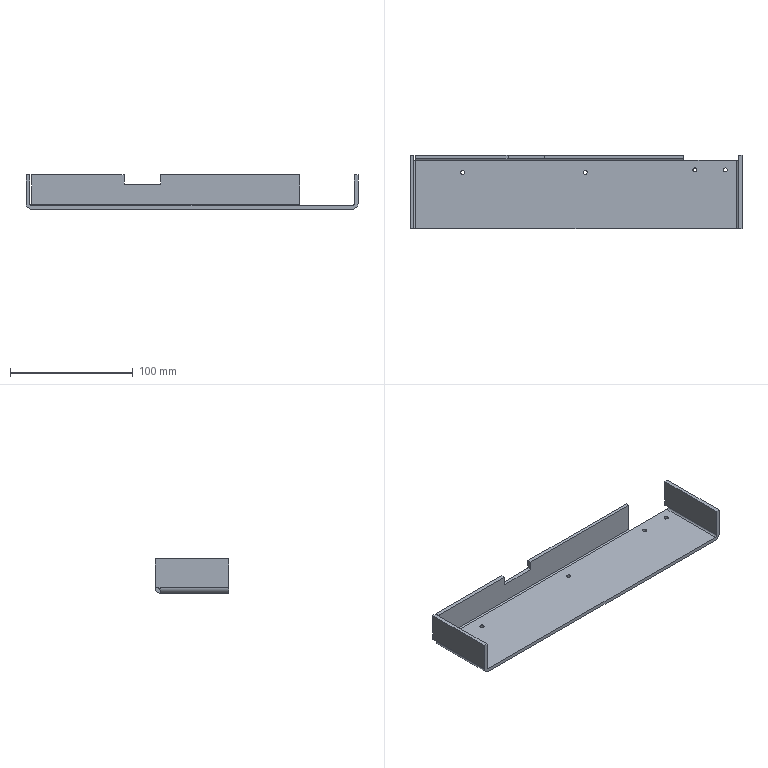Part | NX | features BREP 1 | 1 solid | 34 faces | box 271 x 60 x 28 mm | volume 71630 mm3 | plane 24 | cylinder 10 | commonest cylinder face diameters 3.3 x4 3 x2 9 x2 2 x1 8 x1
STEP:
#1=CARTESIAN_POINT('',(139.15,18.,0.));
#2=VERTEX_POINT('',#1);
#3=CARTESIAN_POINT('',(137.5,18.,0.));
#4=DIRECTION('',(0.,0.,1.));
#5=DIRECTION('',(1.,0.,0.));
#6=AXIS2_PLACEMENT_3D('',#3,#4,#5);
#7=CIRCLE('',#6,1.65);
#8=EDGE_CURVE('',#2,#2,#7,.T.);
#9=ORIENTED_EDGE('',*,*,#8,.T.);
#10=EDGE_LOOP('',(#9));
#11=FACE_BOUND('',#10,.T.);
#12=CARTESIAN_POINT('',(139.15,18.,-3.));
#13=VERTEX_POINT('',#12);
#14=CARTESIAN_POINT('',(137.5,18.,-3.));
#15=DIRECTION('',(0.,0.,1.));
#16=DIRECTION('',(1.,0.,0.));
#17=AXIS2_PLACEMENT_3D('',#14,#15,#16);
#18=CIRCLE('',#17,1.65);
#19=EDGE_CURVE('',#13,#13,#18,.T.);
#20=ORIENTED_EDGE('',*,*,#19,.F.);
#21=EDGE_LOOP('',(#20));
#22=FACE_BOUND('',#21,.T.);
#23=CARTESIAN_POINT('',(137.5,18.,0.));
#24=DIRECTION('',(0.,0.,1.));
#25=DIRECTION('',(1.,0.,0.));
#26=AXIS2_PLACEMENT_3D('',#23,#24,#25);
#27=CYLINDRICAL_SURFACE('',#26,1.65);
#28=ADVANCED_FACE('',(#11,#22),#27,.F.);
#29=CARTESIAN_POINT('',(164.15,18.,0.));
#30=VERTEX_POINT('',#29);
#31=CARTESIAN_POINT('',(162.5,18.,0.));
#32=DIRECTION('',(0.,0.,1.));
#33=DIRECTION('',(1.,0.,0.));
#34=AXIS2_PLACEMENT_3D('',#31,#32,#33);
#35=CIRCLE('',#34,1.65);
#36=EDGE_CURVE('',#30,#30,#35,.T.);
#37=ORIENTED_EDGE('',*,*,#36,.T.);
#38=EDGE_LOOP('',(#37));
#39=FACE_BOUND('',#38,.T.);
#40=CARTESIAN_POINT('',(164.15,18.,-3.));
#41=VERTEX_POINT('',#40);
#42=CARTESIAN_POINT('',(162.5,18.,-3.));
#43=DIRECTION('',(0.,0.,1.));
#44=DIRECTION('',(1.,0.,0.));
#45=AXIS2_PLACEMENT_3D('',#42,#43,#44);
#46=CIRCLE('',#45,1.65);
#47=EDGE_CURVE('',#41,#41,#46,.T.);
#48=ORIENTED_EDGE('',*,*,#47,.F.);
#49=EDGE_LOOP('',(#48));
#50=FACE_BOUND('',#49,.T.);
#51=CARTESIAN_POINT('',(162.5,18.,0.));
#52=DIRECTION('',(0.,0.,1.));
#53=DIRECTION('',(1.,0.,0.));
#54=AXIS2_PLACEMENT_3D('',#51,#52,#53);
#55=CYLINDRICAL_SURFACE('',#54,1.65);
#56=ADVANCED_FACE('',(#39,#50),#55,.F.);
#57=CARTESIAN_POINT('',(49.65,16.,0.));
#58=VERTEX_POINT('',#57);
#59=CARTESIAN_POINT('',(48.,16.,0.));
#60=DIRECTION('',(0.,0.,1.));
#61=DIRECTION('',(1.,0.,0.));
#62=AXIS2_PLACEMENT_3D('',#59,#60,#61);
#63=CIRCLE('',#62,1.65);
#64=EDGE_CURVE('',#58,#58,#63,.T.);
#65=ORIENTED_EDGE('',*,*,#64,.T.);
#66=EDGE_LOOP('',(#65));
#67=FACE_BOUND('',#66,.T.);
#68=CARTESIAN_POINT('',(49.65,16.,-3.));
#69=VERTEX_POINT('',#68);
#70=CARTESIAN_POINT('',(48.,16.,-3.));
#71=DIRECTION('',(0.,0.,1.));
#72=DIRECTION('',(1.,0.,0.));
#73=AXIS2_PLACEMENT_3D('',#70,#71,#72);
#74=CIRCLE('',#73,1.65);
#75=EDGE_CURVE('',#69,#69,#74,.T.);
#76=ORIENTED_EDGE('',*,*,#75,.F.);
#77=EDGE_LOOP('',(#76));
#78=FACE_BOUND('',#77,.T.);
#79=CARTESIAN_POINT('',(48.,16.,0.));
#80=DIRECTION('',(0.,0.,1.));
#81=DIRECTION('',(1.,0.,0.));
#82=AXIS2_PLACEMENT_3D('',#79,#80,#81);
#83=CYLINDRICAL_SURFACE('',#82,1.65);
#84=ADVANCED_FACE('',(#67,#78),#83,.F.);
#85=CARTESIAN_POINT('',(-50.35,16.,0.));
#86=VERTEX_POINT('',#85);
#87=CARTESIAN_POINT('',(-52.,16.,0.));
#88=DIRECTION('',(0.,0.,1.));
#89=DIRECTION('',(1.,0.,0.));
#90=AXIS2_PLACEMENT_3D('',#87,#88,#89);
#91=CIRCLE('',#90,1.65);
#92=EDGE_CURVE('',#86,#86,#91,.T.);
#93=ORIENTED_EDGE('',*,*,#92,.T.);
#94=EDGE_LOOP('',(#93));
#95=FACE_BOUND('',#94,.T.);
#96=CARTESIAN_POINT('',(-50.35,16.,-3.));
#97=VERTEX_POINT('',#96);
#98=CARTESIAN_POINT('',(-52.,16.,-3.));
#99=DIRECTION('',(0.,0.,1.));
#100=DIRECTION('',(1.,0.,0.));
#101=AXIS2_PLACEMENT_3D('',#98,#99,#100);
#102=CIRCLE('',#101,1.65);
#103=EDGE_CURVE('',#97,#97,#102,.T.);
#104=ORIENTED_EDGE('',*,*,#103,.F.);
#105=EDGE_LOOP('',(#104));
#106=FACE_BOUND('',#105,.T.);
#107=CARTESIAN_POINT('',(-52.,16.,0.));
#108=DIRECTION('',(0.,0.,1.));
#109=DIRECTION('',(1.,0.,0.));
#110=AXIS2_PLACEMENT_3D('',#107,#108,#109);
#111=CYLINDRICAL_SURFACE('',#110,1.65);
#112=ADVANCED_FACE('',(#95,#106),#111,.F.);
#113=CARTESIAN_POINT('',(128.5,30.,1.));
#114=VERTEX_POINT('',#113);
#115=CARTESIAN_POINT('',(-90.5,30.,1.));
#116=VERTEX_POINT('',#115);
#117=CARTESIAN_POINT('',(0.,30.,1.));
#118=DIRECTION('',(-1.,0.,0.));
#119=VECTOR('',#118,1000.);
#120=LINE('',#117,#119);
#121=EDGE_CURVE('',#114,#116,#120,.T.);
#122=ORIENTED_EDGE('',*,*,#121,.F.);
#123=CARTESIAN_POINT('',(128.5,26.,-3.));
#124=VERTEX_POINT('',#123);
#125=CARTESIAN_POINT('',(128.5,26.,1.));
#126=DIRECTION('',(1.,0.,0.));
#127=DIRECTION('',(0.,-1.,0.));
#128=AXIS2_PLACEMENT_3D('',#125,#126,#127);
#129=CIRCLE('',#128,4.);
#130=EDGE_CURVE('',#124,#114,#129,.T.);
#131=ORIENTED_EDGE('',*,*,#130,.F.);
#132=CARTESIAN_POINT('',(-90.5,26.,-3.));
#133=VERTEX_POINT('',#132);
#134=CARTESIAN_POINT('',(-90.5,26.,-3.));
#135=DIRECTION('',(1.,0.,0.));
#136=VECTOR('',#135,1000.);
#137=LINE('',#134,#136);
#138=EDGE_CURVE('',#133,#124,#137,.T.);
#139=ORIENTED_EDGE('',*,*,#138,.F.);
#140=CARTESIAN_POINT('',(-90.5,26.,1.));
#141=DIRECTION('',(-1.,0.,0.));
#142=DIRECTION('',(0.,-1.,0.));
#143=AXIS2_PLACEMENT_3D('',#140,#141,#142);
#144=CIRCLE('',#143,4.);
#145=EDGE_CURVE('',#116,#133,#144,.T.);
#146=ORIENTED_EDGE('',*,*,#145,.F.);
#147=EDGE_LOOP('',(#122,#131,#139,#146));
#148=FACE_BOUND('',#147,.T.);
#149=CARTESIAN_POINT('',(-90.5,26.,1.));
#150=DIRECTION('',(-1.,0.,0.));
#151=DIRECTION('',(0.,1.,0.));
#152=AXIS2_PLACEMENT_3D('',#149,#150,#151);
#153=CYLINDRICAL_SURFACE('',#152,4.);
#154=ADVANCED_FACE('',(#148),#153,.T.);
#155=CARTESIAN_POINT('',(128.5,26.,0.));
#156=VERTEX_POINT('',#155);
#157=CARTESIAN_POINT('',(128.5,27.,1.));
#158=VERTEX_POINT('',#157);
#159=CARTESIAN_POINT('',(128.5,26.,1.));
#160=DIRECTION('',(1.,0.,0.));
#161=DIRECTION('',(0.,0.,1.));
#162=AXIS2_PLACEMENT_3D('',#159,#160,#161);
#163=CIRCLE('',#162,1.);
#164=EDGE_CURVE('',#156,#158,#163,.T.);
#165=ORIENTED_EDGE('',*,*,#164,.T.);
#166=CARTESIAN_POINT('',(-90.5,27.,1.));
#167=VERTEX_POINT('',#166);
#168=CARTESIAN_POINT('',(171.5,27.,1.));
#169=DIRECTION('',(-1.,0.,0.));
#170=VECTOR('',#169,1000.);
#171=LINE('',#168,#170);
#172=EDGE_CURVE('',#158,#167,#171,.T.);
#173=ORIENTED_EDGE('',*,*,#172,.T.);
#174=CARTESIAN_POINT('',(-90.5,26.,0.));
#175=VERTEX_POINT('',#174);
#176=CARTESIAN_POINT('',(-90.5,26.,1.));
#177=DIRECTION('',(-1.,0.,0.));
#178=DIRECTION('',(0.,-1.,0.));
#179=AXIS2_PLACEMENT_3D('',#176,#177,#178);
#180=CIRCLE('',#179,1.);
#181=EDGE_CURVE('',#167,#175,#180,.T.);
#182=ORIENTED_EDGE('',*,*,#181,.T.);
#183=CARTESIAN_POINT('',(-90.5,26.,0.));
#184=DIRECTION('',(1.,0.,0.));
#185=VECTOR('',#184,1000.);
#186=LINE('',#183,#185);
#187=EDGE_CURVE('',#175,#156,#186,.T.);
#188=ORIENTED_EDGE('',*,*,#187,.T.);
#189=EDGE_LOOP('',(#165,#173,#182,#188));
#190=FACE_BOUND('',#189,.T.);
#191=CARTESIAN_POINT('',(-90.5,26.,1.));
#192=DIRECTION('',(-1.,0.,0.));
#193=DIRECTION('',(0.,1.,0.));
#194=AXIS2_PLACEMENT_3D('',#191,#192,#193);
#195=CYLINDRICAL_SURFACE('',#194,1.);
#196=ADVANCED_FACE('',(#190),#195,.F.);
#197=CARTESIAN_POINT('',(128.5,30.,25.));
#198=VERTEX_POINT('',#197);
#199=CARTESIAN_POINT('',(15.,30.,25.));
#200=VERTEX_POINT('',#199);
#201=CARTESIAN_POINT('',(-90.5,30.,25.));
#202=DIRECTION('',(-1.,0.,0.));
#203=VECTOR('',#202,1000.);
#204=LINE('',#201,#203);
#205=EDGE_CURVE('',#198,#200,#204,.T.);
#206=ORIENTED_EDGE('',*,*,#205,.F.);
#207=CARTESIAN_POINT('',(128.5,30.,0.));
#208=DIRECTION('',(0.,0.,1.));
#209=VECTOR('',#208,1000.);
#210=LINE('',#207,#209);
#211=EDGE_CURVE('',#114,#198,#210,.T.);
#212=ORIENTED_EDGE('',*,*,#211,.F.);
#213=ORIENTED_EDGE('',*,*,#121,.T.);
#214=CARTESIAN_POINT('',(-90.5,30.,25.));
#215=VERTEX_POINT('',#214);
#216=CARTESIAN_POINT('',(-90.5,30.,0.));
#217=DIRECTION('',(0.,0.,-1.));
#218=VECTOR('',#217,1000.);
#219=LINE('',#216,#218);
#220=EDGE_CURVE('',#215,#116,#219,.T.);
#221=ORIENTED_EDGE('',*,*,#220,.F.);
#222=CARTESIAN_POINT('',(-15.,30.,25.));
#223=VERTEX_POINT('',#222);
#224=CARTESIAN_POINT('',(-90.5,30.,25.));
#225=DIRECTION('',(-1.,0.,0.));
#226=VECTOR('',#225,1000.);
#227=LINE('',#224,#226);
#228=EDGE_CURVE('',#223,#215,#227,.T.);
#229=ORIENTED_EDGE('',*,*,#228,.F.);
#230=CARTESIAN_POINT('',(-15.,30.,17.5));
#231=VERTEX_POINT('',#230);
#232=CARTESIAN_POINT('',(-15.,30.,17.5));
#233=DIRECTION('',(0.,0.,1.));
#234=VECTOR('',#233,1000.);
#235=LINE('',#232,#234);
#236=EDGE_CURVE('',#231,#223,#235,.T.);
#237=ORIENTED_EDGE('',*,*,#236,.F.);
#238=CARTESIAN_POINT('',(15.,30.,17.5));
#239=VERTEX_POINT('',#238);
#240=CARTESIAN_POINT('',(15.,30.,17.5));
#241=DIRECTION('',(-1.,0.,0.));
#242=VECTOR('',#241,1000.);
#243=LINE('',#240,#242);
#244=EDGE_CURVE('',#239,#231,#243,.T.);
#245=ORIENTED_EDGE('',*,*,#244,.F.);
#246=CARTESIAN_POINT('',(15.,30.,17.5));
#247=DIRECTION('',(0.,0.,-1.));
#248=VECTOR('',#247,1000.);
#249=LINE('',#246,#248);
#250=EDGE_CURVE('',#200,#239,#249,.T.);
#251=ORIENTED_EDGE('',*,*,#250,.F.);
#252=EDGE_LOOP('',(#206,#212,#213,#221,#229,#237,#245,#251));
#253=FACE_BOUND('',#252,.T.);
#254=CARTESIAN_POINT('',(0.,30.,0.));
#255=DIRECTION('',(0.,1.,0.));
#256=DIRECTION('',(-1.,0.,0.));
#257=AXIS2_PLACEMENT_3D('',#254,#255,#256);
#258=PLANE('',#257);
#259=ADVANCED_FACE('',(#253),#258,.T.);
#260=CARTESIAN_POINT('',(128.5,27.,25.));
#261=VERTEX_POINT('',#260);
#262=CARTESIAN_POINT('',(128.5,27.,0.));
#263=DIRECTION('',(0.,0.,1.));
#264=VECTOR('',#263,1000.);
#265=LINE('',#262,#264);
#266=EDGE_CURVE('',#158,#261,#265,.T.);
#267=ORIENTED_EDGE('',*,*,#266,.T.);
#268=CARTESIAN_POINT('',(15.,27.,25.));
#269=VERTEX_POINT('',#268);
#270=CARTESIAN_POINT('',(0.,27.,25.));
#271=DIRECTION('',(-1.,0.,0.));
#272=VECTOR('',#271,1000.);
#273=LINE('',#270,#272);
#274=EDGE_CURVE('',#261,#269,#273,.T.);
#275=ORIENTED_EDGE('',*,*,#274,.T.);
#276=CARTESIAN_POINT('',(15.,27.,17.5));
#277=VERTEX_POINT('',#276);
#278=CARTESIAN_POINT('',(15.,27.,0.));
#279=DIRECTION('',(0.,0.,-1.));
#280=VECTOR('',#279,1000.);
#281=LINE('',#278,#280);
#282=EDGE_CURVE('',#269,#277,#281,.T.);
#283=ORIENTED_EDGE('',*,*,#282,.T.);
#284=CARTESIAN_POINT('',(-15.,27.,17.5));
#285=VERTEX_POINT('',#284);
#286=CARTESIAN_POINT('',(0.,27.,17.5));
#287=DIRECTION('',(-1.,0.,0.));
#288=VECTOR('',#287,1000.);
#289=LINE('',#286,#288);
#290=EDGE_CURVE('',#277,#285,#289,.T.);
#291=ORIENTED_EDGE('',*,*,#290,.T.);
#292=CARTESIAN_POINT('',(-15.,27.,25.));
#293=VERTEX_POINT('',#292);
#294=CARTESIAN_POINT('',(-15.,27.,0.));
#295=DIRECTION('',(0.,0.,1.));
#296=VECTOR('',#295,1000.);
#297=LINE('',#294,#296);
#298=EDGE_CURVE('',#285,#293,#297,.T.);
#299=ORIENTED_EDGE('',*,*,#298,.T.);
#300=CARTESIAN_POINT('',(-90.5,27.,25.));
#301=VERTEX_POINT('',#300);
#302=CARTESIAN_POINT('',(0.,27.,25.));
#303=DIRECTION('',(-1.,0.,0.));
#304=VECTOR('',#303,1000.);
#305=LINE('',#302,#304);
#306=EDGE_CURVE('',#293,#301,#305,.T.);
#307=ORIENTED_EDGE('',*,*,#306,.T.);
#308=CARTESIAN_POINT('',(-90.5,27.,0.));
#309=DIRECTION('',(0.,0.,-1.));
#310=VECTOR('',#309,1000.);
#311=LINE('',#308,#310);
#312=EDGE_CURVE('',#301,#167,#311,.T.);
#313=ORIENTED_EDGE('',*,*,#312,.T.);
#314=ORIENTED_EDGE('',*,*,#172,.F.);
#315=EDGE_LOOP('',(#267,#275,#283,#291,#299,#307,#313,#314));
#316=FACE_BOUND('',#315,.T.);
#317=CARTESIAN_POINT('',(0.,27.,0.));
#318=DIRECTION('',(0.,1.,0.));
#319=DIRECTION('',(-1.,0.,0.));
#320=AXIS2_PLACEMENT_3D('',#317,#318,#319);
#321=PLANE('',#320);
#322=ADVANCED_FACE('',(#316),#321,.F.);
#323=ORIENTED_EDGE('',*,*,#274,.F.);
#324=CARTESIAN_POINT('',(128.5,27.,25.));
#325=DIRECTION('',(0.,1.,0.));
#326=VECTOR('',#325,1000.);
#327=LINE('',#324,#326);
#328=EDGE_CURVE('',#261,#198,#327,.T.);
#329=ORIENTED_EDGE('',*,*,#328,.T.);
#330=ORIENTED_EDGE('',*,*,#205,.T.);
#331=CARTESIAN_POINT('',(15.,30.,25.));
#332=DIRECTION('',(0.,1.,0.));
#333=VECTOR('',#332,1000.);
#334=LINE('',#331,#333);
#335=EDGE_CURVE('',#269,#200,#334,.T.);
#336=ORIENTED_EDGE('',*,*,#335,.F.);
#337=EDGE_LOOP('',(#323,#329,#330,#336));
#338=FACE_BOUND('',#337,.T.);
#339=CARTESIAN_POINT('',(-90.5,30.,25.));
#340=DIRECTION('',(0.,0.,1.));
#341=DIRECTION('',(0.,-1.,0.));
#342=AXIS2_PLACEMENT_3D('',#339,#340,#341);
#343=PLANE('',#342);
#344=ADVANCED_FACE('',(#338),#343,.T.);
#345=CARTESIAN_POINT('',(-15.,30.,25.));
#346=DIRECTION('',(0.,-1.,0.));
#347=VECTOR('',#346,1000.);
#348=LINE('',#345,#347);
#349=EDGE_CURVE('',#223,#293,#348,.T.);
#350=ORIENTED_EDGE('',*,*,#349,.F.);
#351=ORIENTED_EDGE('',*,*,#228,.T.);
#352=CARTESIAN_POINT('',(-90.5,30.,25.));
#353=DIRECTION('',(0.,-1.,0.));
#354=VECTOR('',#353,1000.);
#355=LINE('',#352,#354);
#356=EDGE_CURVE('',#215,#301,#355,.T.);
#357=ORIENTED_EDGE('',*,*,#356,.T.);
#358=ORIENTED_EDGE('',*,*,#306,.F.);
#359=EDGE_LOOP('',(#350,#351,#357,#358));
#360=FACE_BOUND('',#359,.T.);
#361=CARTESIAN_POINT('',(-90.5,30.,25.));
#362=DIRECTION('',(0.,0.,1.));
#363=DIRECTION('',(0.,-1.,0.));
#364=AXIS2_PLACEMENT_3D('',#361,#362,#363);
#365=PLANE('',#364);
#366=ADVANCED_FACE('',(#360),#365,.T.);
#367=CARTESIAN_POINT('',(-95.,26.,1.5));
#368=VERTEX_POINT('',#367);
#369=CARTESIAN_POINT('',(-92.,26.,1.5));
#370=VERTEX_POINT('',#369);
#371=CARTESIAN_POINT('',(-95.,26.,1.5));
#372=DIRECTION('',(1.,0.,0.));
#373=VECTOR('',#372,1000.);
#374=LINE('',#371,#373);
#375=EDGE_CURVE('',#368,#370,#374,.T.);
#376=ORIENTED_EDGE('',*,*,#375,.F.);
#377=CARTESIAN_POINT('',(-95.,30.,1.5));
#378=VERTEX_POINT('',#377);
#379=CARTESIAN_POINT('',(-95.,30.,1.5));
#380=DIRECTION('',(0.,1.,0.));
#381=VECTOR('',#380,1000.);
#382=LINE('',#379,#381);
#383=EDGE_CURVE('',#368,#378,#382,.T.);
#384=ORIENTED_EDGE('',*,*,#383,.T.);
#385=CARTESIAN_POINT('',(-92.,30.,1.5));
#386=VERTEX_POINT('',#385);
#387=CARTESIAN_POINT('',(-95.,30.,1.5));
#388=DIRECTION('',(-1.,0.,0.));
#389=VECTOR('',#388,1000.);
#390=LINE('',#387,#389);
#391=EDGE_CURVE('',#386,#378,#390,.T.);
#392=ORIENTED_EDGE('',*,*,#391,.F.);
#393=CARTESIAN_POINT('',(-92.,30.,1.5));
#394=DIRECTION('',(0.,-1.,0.));
#395=VECTOR('',#394,1000.);
#396=LINE('',#393,#395);
#397=EDGE_CURVE('',#386,#370,#396,.T.);
#398=ORIENTED_EDGE('',*,*,#397,.T.);
#399=EDGE_LOOP('',(#376,#384,#392,#398));
#400=FACE_BOUND('',#399,.T.);
#401=CARTESIAN_POINT('',(0.,0.,1.5));
#402=DIRECTION('',(0.,0.,-1.));
#403=DIRECTION('',(-1.,0.,0.));
#404=AXIS2_PLACEMENT_3D('',#401,#402,#403);
#405=PLANE('',#404);
#406=ADVANCED_FACE('',(#400),#405,.T.);
#407=CARTESIAN_POINT('',(-95.,-30.,1.5));
#408=VERTEX_POINT('',#407);
#409=CARTESIAN_POINT('',(-95.,30.,1.5));
#410=DIRECTION('',(0.,1.,0.));
#411=VECTOR('',#410,1000.);
#412=LINE('',#409,#411);
#413=EDGE_CURVE('',#408,#368,#412,.T.);
#414=ORIENTED_EDGE('',*,*,#413,.T.);
#415=CARTESIAN_POINT('',(-90.5,26.,1.5));
#416=DIRECTION('',(0.,-1.,0.));
#417=DIRECTION('',(0.,0.,1.));
#418=AXIS2_PLACEMENT_3D('',#415,#416,#417);
#419=CIRCLE('',#418,4.5);
#420=EDGE_CURVE('',#368,#133,#419,.T.);
#421=ORIENTED_EDGE('',*,*,#420,.T.);
#422=CARTESIAN_POINT('',(-90.5,-30.,-3.));
#423=VERTEX_POINT('',#422);
#424=CARTESIAN_POINT('',(-90.5,-30.,-3.));
#425=DIRECTION('',(0.,1.,0.));
#426=VECTOR('',#425,1000.);
#427=LINE('',#424,#426);
#428=EDGE_CURVE('',#423,#133,#427,.T.);
#429=ORIENTED_EDGE('',*,*,#428,.F.);
#430=CARTESIAN_POINT('',(-90.5,-30.,1.5));
#431=DIRECTION('',(0.,-1.,0.));
#432=DIRECTION('',(0.,0.,-1.));
#433=AXIS2_PLACEMENT_3D('',#430,#431,#432);
#434=CIRCLE('',#433,4.5);
#435=EDGE_CURVE('',#408,#423,#434,.T.);
#436=ORIENTED_EDGE('',*,*,#435,.F.);
#437=EDGE_LOOP('',(#414,#421,#429,#436));
#438=FACE_BOUND('',#437,.T.);
#439=CARTESIAN_POINT('',(-90.5,-30.,1.5));
#440=DIRECTION('',(0.,-1.,0.));
#441=DIRECTION('',(-1.,0.,0.));
#442=AXIS2_PLACEMENT_3D('',#439,#440,#441);
#443=CYLINDRICAL_SURFACE('',#442,4.5);
#444=ADVANCED_FACE('',(#438),#443,.T.);
#445=CARTESIAN_POINT('',(173.,26.,1.5));
#446=VERTEX_POINT('',#445);
#447=CARTESIAN_POINT('',(176.,26.,1.5));
#448=VERTEX_POINT('',#447);
#449=CARTESIAN_POINT('',(173.,26.,1.5));
#450=DIRECTION('',(1.,0.,0.));
#451=VECTOR('',#450,1000.);
#452=LINE('',#449,#451);
#453=EDGE_CURVE('',#446,#448,#452,.T.);
#454=ORIENTED_EDGE('',*,*,#453,.F.);
#455=CARTESIAN_POINT('',(173.,30.,1.5));
#456=VERTEX_POINT('',#455);
#457=CARTESIAN_POINT('',(173.,-30.,1.5));
#458=DIRECTION('',(0.,1.,0.));
#459=VECTOR('',#458,1000.);
#460=LINE('',#457,#459);
#461=EDGE_CURVE('',#446,#456,#460,.T.);
#462=ORIENTED_EDGE('',*,*,#461,.T.);
#463=CARTESIAN_POINT('',(176.,30.,1.5));
#464=VERTEX_POINT('',#463);
#465=CARTESIAN_POINT('',(173.,30.,1.5));
#466=DIRECTION('',(1.,0.,0.));
#467=VECTOR('',#466,1000.);
#468=LINE('',#465,#467);
#469=EDGE_CURVE('',#456,#464,#468,.T.);
#470=ORIENTED_EDGE('',*,*,#469,.T.);
#471=CARTESIAN_POINT('',(176.,-30.,1.5));
#472=DIRECTION('',(0.,-1.,0.));
#473=VECTOR('',#472,1000.);
#474=LINE('',#471,#473);
#475=EDGE_CURVE('',#464,#448,#474,.T.);
#476=ORIENTED_EDGE('',*,*,#475,.T.);
#477=EDGE_LOOP('',(#454,#462,#470,#476));
#478=FACE_BOUND('',#477,.T.);
#479=CARTESIAN_POINT('',(0.,0.,1.5));
#480=DIRECTION('',(0.,0.,1.));
#481=DIRECTION('',(1.,0.,0.));
#482=AXIS2_PLACEMENT_3D('',#479,#480,#481);
#483=PLANE('',#482);
#484=ADVANCED_FACE('',(#478),#483,.F.);
#485=CARTESIAN_POINT('',(171.5,26.,-3.));
#486=VERTEX_POINT('',#485);
#487=CARTESIAN_POINT('',(171.5,-30.,-3.));
#488=VERTEX_POINT('',#487);
#489=CARTESIAN_POINT('',(171.5,30.,-3.));
#490=DIRECTION('',(0.,-1.,0.));
#491=VECTOR('',#490,1000.);
#492=LINE('',#489,#491);
#493=EDGE_CURVE('',#486,#488,#492,.T.);
#494=ORIENTED_EDGE('',*,*,#493,.F.);
#495=CARTESIAN_POINT('',(171.5,26.,1.5));
#496=DIRECTION('',(0.,-1.,0.));
#497=DIRECTION('',(0.,0.,1.));
#498=AXIS2_PLACEMENT_3D('',#495,#496,#497);
#499=CIRCLE('',#498,4.5);
#500=EDGE_CURVE('',#486,#448,#499,.T.);
#501=ORIENTED_EDGE('',*,*,#500,.T.);
#502=CARTESIAN_POINT('',(176.,-30.,1.5));
#503=VERTEX_POINT('',#502);
#504=CARTESIAN_POINT('',(176.,-30.,1.5));
#505=DIRECTION('',(0.,-1.,0.));
#506=VECTOR('',#505,1000.);
#507=LINE('',#504,#506);
#508=EDGE_CURVE('',#448,#503,#507,.T.);
#509=ORIENTED_EDGE('',*,*,#508,.T.);
#510=CARTESIAN_POINT('',(171.5,-30.,1.5));
#511=DIRECTION('',(0.,-1.,0.));
#512=DIRECTION('',(0.,0.,1.));
#513=AXIS2_PLACEMENT_3D('',#510,#511,#512);
#514=CIRCLE('',#513,4.5);
#515=EDGE_CURVE('',#488,#503,#514,.T.);
#516=ORIENTED_EDGE('',*,*,#515,.F.);
#517=EDGE_LOOP('',(#494,#501,#509,#516));
#518=FACE_BOUND('',#517,.T.);
#519=CARTESIAN_POINT('',(171.5,30.,1.5));
#520=DIRECTION('',(0.,1.,0.));
#521=DIRECTION('',(1.,0.,0.));
#522=AXIS2_PLACEMENT_3D('',#519,#520,#521);
#523=CYLINDRICAL_SURFACE('',#522,4.5);
#524=ADVANCED_FACE('',(#518),#523,.T.);
#525=CARTESIAN_POINT('',(171.5,26.,0.));
#526=VERTEX_POINT('',#525);
#527=CARTESIAN_POINT('',(171.5,26.,1.5));
#528=DIRECTION('',(0.,-1.,0.));
#529=DIRECTION('',(0.,0.,1.));
#530=AXIS2_PLACEMENT_3D('',#527,#528,#529);
#531=CIRCLE('',#530,1.5);
#532=EDGE_CURVE('',#526,#446,#531,.T.);
#533=ORIENTED_EDGE('',*,*,#532,.T.);
#534=ORIENTED_EDGE('',*,*,#453,.T.);
#535=ORIENTED_EDGE('',*,*,#500,.F.);
#536=CARTESIAN_POINT('',(-90.5,26.,-3.));
#537=DIRECTION('',(1.,0.,0.));
#538=VECTOR('',#537,1000.);
#539=LINE('',#536,#538);
#540=EDGE_CURVE('',#124,#486,#539,.T.);
#541=ORIENTED_EDGE('',*,*,#540,.F.);
#542=CARTESIAN_POINT('',(128.5,26.,0.));
#543=DIRECTION('',(0.,0.,-1.));
#544=VECTOR('',#543,1000.);
#545=LINE('',#542,#544);
#546=EDGE_CURVE('',#156,#124,#545,.T.);
#547=ORIENTED_EDGE('',*,*,#546,.F.);
#548=CARTESIAN_POINT('',(-90.5,26.,0.));
#549=DIRECTION('',(1.,0.,0.));
#550=VECTOR('',#549,1000.);
#551=LINE('',#548,#550);
#552=EDGE_CURVE('',#156,#526,#551,.T.);
#553=ORIENTED_EDGE('',*,*,#552,.T.);
#554=EDGE_LOOP('',(#533,#534,#535,#541,#547,#553));
#555=FACE_BOUND('',#554,.T.);
#556=CARTESIAN_POINT('',(171.5,26.,1.5));
#557=DIRECTION('',(0.,1.,0.));
#558=DIRECTION('',(0.,0.,1.));
#559=AXIS2_PLACEMENT_3D('',#556,#557,#558);
#560=PLANE('',#559);
#561=ADVANCED_FACE('',(#555),#560,.T.);
#562=ORIENTED_EDGE('',*,*,#19,.T.);
#563=EDGE_LOOP('',(#562));
#564=FACE_BOUND('',#563,.T.);
#565=ORIENTED_EDGE('',*,*,#47,.T.);
#566=EDGE_LOOP('',(#565));
#567=FACE_BOUND('',#566,.T.);
#568=ORIENTED_EDGE('',*,*,#75,.T.);
#569=EDGE_LOOP('',(#568));
#570=FACE_BOUND('',#569,.T.);
#571=ORIENTED_EDGE('',*,*,#103,.T.);
#572=EDGE_LOOP('',(#571));
#573=FACE_BOUND('',#572,.T.);
#574=ORIENTED_EDGE('',*,*,#428,.T.);
#575=ORIENTED_EDGE('',*,*,#138,.T.);
#576=ORIENTED_EDGE('',*,*,#540,.T.);
#577=ORIENTED_EDGE('',*,*,#493,.T.);
#578=CARTESIAN_POINT('',(-95.,-30.,-3.));
#579=DIRECTION('',(1.,0.,0.));
#580=VECTOR('',#579,1000.);
#581=LINE('',#578,#580);
#582=EDGE_CURVE('',#423,#488,#581,.T.);
#583=ORIENTED_EDGE('',*,*,#582,.F.);
#584=EDGE_LOOP('',(#574,#575,#576,#577,#583));
#585=FACE_BOUND('',#584,.T.);
#586=CARTESIAN_POINT('',(0.,0.,-3.));
#587=DIRECTION('',(0.,0.,-1.));
#588=DIRECTION('',(-1.,0.,0.));
#589=AXIS2_PLACEMENT_3D('',#586,#587,#588);
#590=PLANE('',#589);
#591=ADVANCED_FACE('',(#564,#567,#570,#573,#585),#590,.T.);
#592=ORIENTED_EDGE('',*,*,#8,.F.);
#593=EDGE_LOOP('',(#592));
#594=FACE_BOUND('',#593,.T.);
#595=ORIENTED_EDGE('',*,*,#36,.F.);
#596=EDGE_LOOP('',(#595));
#597=FACE_BOUND('',#596,.T.);
#598=ORIENTED_EDGE('',*,*,#64,.F.);
#599=EDGE_LOOP('',(#598));
#600=FACE_BOUND('',#599,.T.);
#601=ORIENTED_EDGE('',*,*,#92,.F.);
#602=EDGE_LOOP('',(#601));
#603=FACE_BOUND('',#602,.T.);
#604=ORIENTED_EDGE('',*,*,#187,.F.);
#605=CARTESIAN_POINT('',(-90.5,-30.,0.));
#606=VERTEX_POINT('',#605);
#607=CARTESIAN_POINT('',(-90.5,-30.,0.));
#608=DIRECTION('',(0.,1.,0.));
#609=VECTOR('',#608,1000.);
#610=LINE('',#607,#609);
#611=EDGE_CURVE('',#606,#175,#610,.T.);
#612=ORIENTED_EDGE('',*,*,#611,.F.);
#613=CARTESIAN_POINT('',(171.5,-30.,0.));
#614=VERTEX_POINT('',#613);
#615=CARTESIAN_POINT('',(-95.,-30.,0.));
#616=DIRECTION('',(1.,0.,0.));
#617=VECTOR('',#616,1000.);
#618=LINE('',#615,#617);
#619=EDGE_CURVE('',#606,#614,#618,.T.);
#620=ORIENTED_EDGE('',*,*,#619,.T.);
#621=CARTESIAN_POINT('',(171.5,30.,0.));
#622=DIRECTION('',(0.,-1.,0.));
#623=VECTOR('',#622,1000.);
#624=LINE('',#621,#623);
#625=EDGE_CURVE('',#526,#614,#624,.T.);
#626=ORIENTED_EDGE('',*,*,#625,.F.);
#627=ORIENTED_EDGE('',*,*,#552,.F.);
#628=EDGE_LOOP('',(#604,#612,#620,#626,#627));
#629=FACE_BOUND('',#628,.T.);
#630=CARTESIAN_POINT('',(0.,0.,0.));
#631=DIRECTION('',(0.,0.,-1.));
#632=DIRECTION('',(-1.,0.,0.));
#633=AXIS2_PLACEMENT_3D('',#630,#631,#632);
#634=PLANE('',#633);
#635=ADVANCED_FACE('',(#594,#597,#600,#603,#629),#634,.F.);
#636=ORIENTED_EDGE('',*,*,#582,.T.);
#637=ORIENTED_EDGE('',*,*,#515,.T.);
#638=CARTESIAN_POINT('',(176.,-30.,25.));
#639=VERTEX_POINT('',#638);
#640=CARTESIAN_POINT('',(176.,-30.,0.));
#641=DIRECTION('',(0.,0.,1.));
#642=VECTOR('',#641,1000.);
#643=LINE('',#640,#642);
#644=EDGE_CURVE('',#503,#639,#643,.T.);
#645=ORIENTED_EDGE('',*,*,#644,.T.);
#646=CARTESIAN_POINT('',(173.,-30.,25.));
#647=VERTEX_POINT('',#646);
#648=CARTESIAN_POINT('',(176.,-30.,25.));
#649=DIRECTION('',(-1.,0.,0.));
#650=VECTOR('',#649,1000.);
#651=LINE('',#648,#650);
#652=EDGE_CURVE('',#639,#647,#651,.T.);
#653=ORIENTED_EDGE('',*,*,#652,.T.);
#654=CARTESIAN_POINT('',(173.,-30.,1.5));
#655=VERTEX_POINT('',#654);
#656=CARTESIAN_POINT('',(173.,-30.,0.));
#657=DIRECTION('',(0.,0.,1.));
#658=VECTOR('',#657,1000.);
#659=LINE('',#656,#658);
#660=EDGE_CURVE('',#655,#647,#659,.T.);
#661=ORIENTED_EDGE('',*,*,#660,.F.);
#662=CARTESIAN_POINT('',(171.5,-30.,1.5));
#663=DIRECTION('',(0.,-1.,0.));
#664=DIRECTION('',(0.,0.,1.));
#665=AXIS2_PLACEMENT_3D('',#662,#663,#664);
#666=CIRCLE('',#665,1.5);
#667=EDGE_CURVE('',#614,#655,#666,.T.);
#668=ORIENTED_EDGE('',*,*,#667,.F.);
#669=ORIENTED_EDGE('',*,*,#619,.F.);
#670=CARTESIAN_POINT('',(-92.,-30.,1.5));
#671=VERTEX_POINT('',#670);
#672=CARTESIAN_POINT('',(-90.5,-30.,1.5));
#673=DIRECTION('',(0.,-1.,0.));
#674=DIRECTION('',(0.,0.,-1.));
#675=AXIS2_PLACEMENT_3D('',#672,#673,#674);
#676=CIRCLE('',#675,1.5);
#677=EDGE_CURVE('',#671,#606,#676,.T.);
#678=ORIENTED_EDGE('',*,*,#677,.F.);
#679=CARTESIAN_POINT('',(-92.,-30.,25.));
#680=VERTEX_POINT('',#679);
#681=CARTESIAN_POINT('',(-92.,-30.,0.));
#682=DIRECTION('',(0.,0.,-1.));
#683=VECTOR('',#682,1000.);
#684=LINE('',#681,#683);
#685=EDGE_CURVE('',#680,#671,#684,.T.);
#686=ORIENTED_EDGE('',*,*,#685,.F.);
#687=CARTESIAN_POINT('',(-95.,-30.,25.));
#688=VERTEX_POINT('',#687);
#689=CARTESIAN_POINT('',(-95.,-30.,25.));
#690=DIRECTION('',(1.,0.,0.));
#691=VECTOR('',#690,1000.);
#692=LINE('',#689,#691);
#693=EDGE_CURVE('',#688,#680,#692,.T.);
#694=ORIENTED_EDGE('',*,*,#693,.F.);
#695=CARTESIAN_POINT('',(-95.,-30.,25.));
#696=DIRECTION('',(0.,0.,-1.));
#697=VECTOR('',#696,1000.);
#698=LINE('',#695,#697);
#699=EDGE_CURVE('',#688,#408,#698,.T.);
#700=ORIENTED_EDGE('',*,*,#699,.T.);
#701=ORIENTED_EDGE('',*,*,#435,.T.);
#702=EDGE_LOOP('',(#636,#637,#645,#653,#661,#668,#669,#678,#686,#694,#700,#701));
#703=FACE_BOUND('',#702,.T.);
#704=CARTESIAN_POINT('',(-95.,-30.,-3.));
#705=DIRECTION('',(0.,-1.,0.));
#706=DIRECTION('',(1.,0.,0.));
#707=AXIS2_PLACEMENT_3D('',#704,#705,#706);
#708=PLANE('',#707);
#709=ADVANCED_FACE('',(#703),#708,.T.);
#710=ORIENTED_EDGE('',*,*,#420,.F.);
#711=ORIENTED_EDGE('',*,*,#375,.T.);
#712=CARTESIAN_POINT('',(-90.5,26.,1.5));
#713=DIRECTION('',(0.,-1.,0.));
#714=DIRECTION('',(0.,0.,1.));
#715=AXIS2_PLACEMENT_3D('',#712,#713,#714);
#716=CIRCLE('',#715,1.5);
#717=EDGE_CURVE('',#370,#175,#716,.T.);
#718=ORIENTED_EDGE('',*,*,#717,.T.);
#719=CARTESIAN_POINT('',(-90.5,26.,0.));
#720=DIRECTION('',(0.,0.,-1.));
#721=VECTOR('',#720,1000.);
#722=LINE('',#719,#721);
#723=EDGE_CURVE('',#175,#133,#722,.T.);
#724=ORIENTED_EDGE('',*,*,#723,.T.);
#725=EDGE_LOOP('',(#710,#711,#718,#724));
#726=FACE_BOUND('',#725,.T.);
#727=CARTESIAN_POINT('',(-90.5,26.,1.5));
#728=DIRECTION('',(0.,1.,0.));
#729=DIRECTION('',(0.,0.,1.));
#730=AXIS2_PLACEMENT_3D('',#727,#728,#729);
#731=PLANE('',#730);
#732=ADVANCED_FACE('',(#726),#731,.T.);
#733=ORIENTED_EDGE('',*,*,#717,.F.);
#734=CARTESIAN_POINT('',(-92.,30.,1.5));
#735=DIRECTION('',(0.,-1.,0.));
#736=VECTOR('',#735,1000.);
#737=LINE('',#734,#736);
#738=EDGE_CURVE('',#370,#671,#737,.T.);
#739=ORIENTED_EDGE('',*,*,#738,.T.);
#740=ORIENTED_EDGE('',*,*,#677,.T.);
#741=ORIENTED_EDGE('',*,*,#611,.T.);
#742=EDGE_LOOP('',(#733,#739,#740,#741));
#743=FACE_BOUND('',#742,.T.);
#744=CARTESIAN_POINT('',(-90.5,-30.,1.5));
#745=DIRECTION('',(0.,-1.,0.));
#746=DIRECTION('',(-1.,0.,0.));
#747=AXIS2_PLACEMENT_3D('',#744,#745,#746);
#748=CYLINDRICAL_SURFACE('',#747,1.5);
#749=ADVANCED_FACE('',(#743),#748,.F.);
#750=CARTESIAN_POINT('',(-92.,30.,25.));
#751=VERTEX_POINT('',#750);
#752=CARTESIAN_POINT('',(-92.,30.,0.));
#753=DIRECTION('',(0.,0.,1.));
#754=VECTOR('',#753,1000.);
#755=LINE('',#752,#754);
#756=EDGE_CURVE('',#386,#751,#755,.T.);
#757=ORIENTED_EDGE('',*,*,#756,.F.);
#758=ORIENTED_EDGE('',*,*,#391,.T.);
#759=CARTESIAN_POINT('',(-95.,30.,25.));
#760=VERTEX_POINT('',#759);
#761=CARTESIAN_POINT('',(-95.,30.,0.));
#762=DIRECTION('',(0.,0.,1.));
#763=VECTOR('',#762,1000.);
#764=LINE('',#761,#763);
#765=EDGE_CURVE('',#378,#760,#764,.T.);
#766=ORIENTED_EDGE('',*,*,#765,.T.);
#767=CARTESIAN_POINT('',(-95.,30.,25.));
#768=DIRECTION('',(1.,0.,0.));
#769=VECTOR('',#768,1000.);
#770=LINE('',#767,#769);
#771=EDGE_CURVE('',#760,#751,#770,.T.);
#772=ORIENTED_EDGE('',*,*,#771,.T.);
#773=EDGE_LOOP('',(#757,#758,#766,#772));
#774=FACE_BOUND('',#773,.T.);
#775=CARTESIAN_POINT('',(-95.,30.,0.));
#776=DIRECTION('',(0.,1.,0.));
#777=DIRECTION('',(0.,0.,1.));
#778=AXIS2_PLACEMENT_3D('',#775,#776,#777);
#779=PLANE('',#778);
#780=ADVANCED_FACE('',(#774),#779,.T.);
#781=ORIENTED_EDGE('',*,*,#413,.F.);
#782=ORIENTED_EDGE('',*,*,#699,.F.);
#783=CARTESIAN_POINT('',(-95.,30.,25.));
#784=DIRECTION('',(0.,-1.,0.));
#785=VECTOR('',#784,1000.);
#786=LINE('',#783,#785);
#787=EDGE_CURVE('',#760,#688,#786,.T.);
#788=ORIENTED_EDGE('',*,*,#787,.F.);
#789=ORIENTED_EDGE('',*,*,#765,.F.);
#790=ORIENTED_EDGE('',*,*,#383,.F.);
#791=EDGE_LOOP('',(#781,#782,#788,#789,#790));
#792=FACE_BOUND('',#791,.T.);
#793=CARTESIAN_POINT('',(-95.,0.,0.));
#794=DIRECTION('',(1.,0.,0.));
#795=DIRECTION('',(0.,0.,-1.));
#796=AXIS2_PLACEMENT_3D('',#793,#794,#795);
#797=PLANE('',#796);
#798=ADVANCED_FACE('',(#792),#797,.F.);
#799=ORIENTED_EDGE('',*,*,#685,.T.);
#800=ORIENTED_EDGE('',*,*,#738,.F.);
#801=ORIENTED_EDGE('',*,*,#397,.F.);
#802=ORIENTED_EDGE('',*,*,#756,.T.);
#803=CARTESIAN_POINT('',(-92.,0.,25.));
#804=DIRECTION('',(0.,-1.,0.));
#805=VECTOR('',#804,1000.);
#806=LINE('',#803,#805);
#807=EDGE_CURVE('',#751,#680,#806,.T.);
#808=ORIENTED_EDGE('',*,*,#807,.T.);
#809=EDGE_LOOP('',(#799,#800,#801,#802,#808));
#810=FACE_BOUND('',#809,.T.);
#811=CARTESIAN_POINT('',(-92.,0.,0.));
#812=DIRECTION('',(1.,0.,0.));
#813=DIRECTION('',(0.,0.,-1.));
#814=AXIS2_PLACEMENT_3D('',#811,#812,#813);
#815=PLANE('',#814);
#816=ADVANCED_FACE('',(#810),#815,.T.);
#817=ORIENTED_EDGE('',*,*,#807,.F.);
#818=ORIENTED_EDGE('',*,*,#771,.F.);
#819=ORIENTED_EDGE('',*,*,#787,.T.);
#820=ORIENTED_EDGE('',*,*,#693,.T.);
#821=EDGE_LOOP('',(#817,#818,#819,#820));
#822=FACE_BOUND('',#821,.T.);
#823=CARTESIAN_POINT('',(-95.,30.,25.));
#824=DIRECTION('',(0.,0.,1.));
#825=DIRECTION('',(1.,0.,0.));
#826=AXIS2_PLACEMENT_3D('',#823,#824,#825);
#827=PLANE('',#826);
#828=ADVANCED_FACE('',(#822),#827,.T.);
#829=ORIENTED_EDGE('',*,*,#532,.F.);
#830=ORIENTED_EDGE('',*,*,#625,.T.);
#831=ORIENTED_EDGE('',*,*,#667,.T.);
#832=CARTESIAN_POINT('',(173.,-30.,1.5));
#833=DIRECTION('',(0.,1.,0.));
#834=VECTOR('',#833,1000.);
#835=LINE('',#832,#834);
#836=EDGE_CURVE('',#655,#446,#835,.T.);
#837=ORIENTED_EDGE('',*,*,#836,.T.);
#838=EDGE_LOOP('',(#829,#830,#831,#837));
#839=FACE_BOUND('',#838,.T.);
#840=CARTESIAN_POINT('',(171.5,30.,1.5));
#841=DIRECTION('',(0.,1.,0.));
#842=DIRECTION('',(1.,0.,0.));
#843=AXIS2_PLACEMENT_3D('',#840,#841,#842);
#844=CYLINDRICAL_SURFACE('',#843,1.5);
#845=ADVANCED_FACE('',(#839),#844,.F.);
#846=CARTESIAN_POINT('',(176.,30.,25.));
#847=VERTEX_POINT('',#846);
#848=CARTESIAN_POINT('',(176.,30.,25.));
#849=DIRECTION('',(0.,0.,-1.));
#850=VECTOR('',#849,1000.);
#851=LINE('',#848,#850);
#852=EDGE_CURVE('',#847,#464,#851,.T.);
#853=ORIENTED_EDGE('',*,*,#852,.T.);
#854=ORIENTED_EDGE('',*,*,#469,.F.);
#855=CARTESIAN_POINT('',(173.,30.,25.));
#856=VERTEX_POINT('',#855);
#857=CARTESIAN_POINT('',(173.,30.,0.));
#858=DIRECTION('',(0.,0.,-1.));
#859=VECTOR('',#858,1000.);
#860=LINE('',#857,#859);
#861=EDGE_CURVE('',#856,#456,#860,.T.);
#862=ORIENTED_EDGE('',*,*,#861,.F.);
#863=CARTESIAN_POINT('',(176.,30.,25.));
#864=DIRECTION('',(-1.,0.,0.));
#865=VECTOR('',#864,1000.);
#866=LINE('',#863,#865);
#867=EDGE_CURVE('',#847,#856,#866,.T.);
#868=ORIENTED_EDGE('',*,*,#867,.F.);
#869=EDGE_LOOP('',(#853,#854,#862,#868));
#870=FACE_BOUND('',#869,.T.);
#871=CARTESIAN_POINT('',(176.,30.,25.));
#872=DIRECTION('',(0.,1.,0.));
#873=DIRECTION('',(0.,0.,1.));
#874=AXIS2_PLACEMENT_3D('',#871,#872,#873);
#875=PLANE('',#874);
#876=ADVANCED_FACE('',(#870),#875,.T.);
#877=ORIENTED_EDGE('',*,*,#475,.F.);
#878=ORIENTED_EDGE('',*,*,#852,.F.);
#879=CARTESIAN_POINT('',(176.,-30.,25.));
#880=DIRECTION('',(0.,1.,0.));
#881=VECTOR('',#880,1000.);
#882=LINE('',#879,#881);
#883=EDGE_CURVE('',#639,#847,#882,.T.);
#884=ORIENTED_EDGE('',*,*,#883,.F.);
#885=ORIENTED_EDGE('',*,*,#644,.F.);
#886=ORIENTED_EDGE('',*,*,#508,.F.);
#887=EDGE_LOOP('',(#877,#878,#884,#885,#886));
#888=FACE_BOUND('',#887,.T.);
#889=CARTESIAN_POINT('',(176.,0.,0.));
#890=DIRECTION('',(-1.,0.,0.));
#891=DIRECTION('',(0.,0.,1.));
#892=AXIS2_PLACEMENT_3D('',#889,#890,#891);
#893=PLANE('',#892);
#894=ADVANCED_FACE('',(#888),#893,.F.);
#895=ORIENTED_EDGE('',*,*,#861,.T.);
#896=ORIENTED_EDGE('',*,*,#461,.F.);
#897=ORIENTED_EDGE('',*,*,#836,.F.);
#898=ORIENTED_EDGE('',*,*,#660,.T.);
#899=CARTESIAN_POINT('',(173.,0.,25.));
#900=DIRECTION('',(0.,1.,0.));
#901=VECTOR('',#900,1000.);
#902=LINE('',#899,#901);
#903=EDGE_CURVE('',#647,#856,#902,.T.);
#904=ORIENTED_EDGE('',*,*,#903,.T.);
#905=EDGE_LOOP('',(#895,#896,#897,#898,#904));
#906=FACE_BOUND('',#905,.T.);
#907=CARTESIAN_POINT('',(173.,0.,0.));
#908=DIRECTION('',(-1.,0.,0.));
#909=DIRECTION('',(0.,0.,1.));
#910=AXIS2_PLACEMENT_3D('',#907,#908,#909);
#911=PLANE('',#910);
#912=ADVANCED_FACE('',(#906),#911,.T.);
#913=ORIENTED_EDGE('',*,*,#903,.F.);
#914=ORIENTED_EDGE('',*,*,#652,.F.);
#915=ORIENTED_EDGE('',*,*,#883,.T.);
#916=ORIENTED_EDGE('',*,*,#867,.T.);
#917=EDGE_LOOP('',(#913,#914,#915,#916));
#918=FACE_BOUND('',#917,.T.);
#919=CARTESIAN_POINT('',(176.,-30.,25.));
#920=DIRECTION('',(0.,0.,1.));
#921=DIRECTION('',(1.,0.,0.));
#922=AXIS2_PLACEMENT_3D('',#919,#920,#921);
#923=PLANE('',#922);
#924=ADVANCED_FACE('',(#918),#923,.T.);
#925=ORIENTED_EDGE('',*,*,#181,.F.);
#926=ORIENTED_EDGE('',*,*,#312,.F.);
#927=ORIENTED_EDGE('',*,*,#356,.F.);
#928=ORIENTED_EDGE('',*,*,#220,.T.);
#929=ORIENTED_EDGE('',*,*,#145,.T.);
#930=ORIENTED_EDGE('',*,*,#723,.F.);
#931=EDGE_LOOP('',(#925,#926,#927,#928,#929,#930));
#932=FACE_BOUND('',#931,.T.);
#933=CARTESIAN_POINT('',(-90.5,26.,1.));
#934=DIRECTION('',(1.,0.,0.));
#935=DIRECTION('',(0.,1.,0.));
#936=AXIS2_PLACEMENT_3D('',#933,#934,#935);
#937=PLANE('',#936);
#938=ADVANCED_FACE('',(#932),#937,.F.);
#939=CARTESIAN_POINT('',(15.,20.,17.5));
#940=DIRECTION('',(0.,1.,0.));
#941=VECTOR('',#940,1000.);
#942=LINE('',#939,#941);
#943=EDGE_CURVE('',#277,#239,#942,.T.);
#944=ORIENTED_EDGE('',*,*,#943,.T.);
#945=ORIENTED_EDGE('',*,*,#244,.T.);
#946=CARTESIAN_POINT('',(-15.,20.,17.5));
#947=DIRECTION('',(0.,1.,0.));
#948=VECTOR('',#947,1000.);
#949=LINE('',#946,#948);
#950=EDGE_CURVE('',#285,#231,#949,.T.);
#951=ORIENTED_EDGE('',*,*,#950,.F.);
#952=ORIENTED_EDGE('',*,*,#290,.F.);
#953=EDGE_LOOP('',(#944,#945,#951,#952));
#954=FACE_BOUND('',#953,.T.);
#955=CARTESIAN_POINT('',(15.,20.,17.5));
#956=DIRECTION('',(0.,0.,-1.));
#957=DIRECTION('',(0.,1.,0.));
#958=AXIS2_PLACEMENT_3D('',#955,#956,#957);
#959=PLANE('',#958);
#960=ADVANCED_FACE('',(#954),#959,.F.);
#961=ORIENTED_EDGE('',*,*,#950,.T.);
#962=ORIENTED_EDGE('',*,*,#236,.T.);
#963=ORIENTED_EDGE('',*,*,#349,.T.);
#964=ORIENTED_EDGE('',*,*,#298,.F.);
#965=EDGE_LOOP('',(#961,#962,#963,#964));
#966=FACE_BOUND('',#965,.T.);
#967=CARTESIAN_POINT('',(-15.,20.,17.5));
#968=DIRECTION('',(-1.,0.,0.));
#969=DIRECTION('',(0.,-1.,0.));
#970=AXIS2_PLACEMENT_3D('',#967,#968,#969);
#971=PLANE('',#970);
#972=ADVANCED_FACE('',(#966),#971,.F.);
#973=ORIENTED_EDGE('',*,*,#335,.T.);
#974=ORIENTED_EDGE('',*,*,#250,.T.);
#975=ORIENTED_EDGE('',*,*,#943,.F.);
#976=ORIENTED_EDGE('',*,*,#282,.F.);
#977=EDGE_LOOP('',(#973,#974,#975,#976));
#978=FACE_BOUND('',#977,.T.);
#979=CARTESIAN_POINT('',(15.,20.,17.5));
#980=DIRECTION('',(1.,0.,0.));
#981=DIRECTION('',(0.,1.,0.));
#982=AXIS2_PLACEMENT_3D('',#979,#980,#981);
#983=PLANE('',#982);
#984=ADVANCED_FACE('',(#978),#983,.F.);
#985=ORIENTED_EDGE('',*,*,#328,.F.);
#986=ORIENTED_EDGE('',*,*,#266,.F.);
#987=ORIENTED_EDGE('',*,*,#164,.F.);
#988=ORIENTED_EDGE('',*,*,#546,.T.);
#989=ORIENTED_EDGE('',*,*,#130,.T.);
#990=ORIENTED_EDGE('',*,*,#211,.T.);
#991=EDGE_LOOP('',(#985,#986,#987,#988,#989,#990));
#992=FACE_BOUND('',#991,.T.);
#993=CARTESIAN_POINT('',(128.5,27.,0.));
#994=DIRECTION('',(-1.,0.,0.));
#995=DIRECTION('',(0.,0.,1.));
#996=AXIS2_PLACEMENT_3D('',#993,#994,#995);
#997=PLANE('',#996);
#998=ADVANCED_FACE('',(#992),#997,.F.);
#999=CLOSED_SHELL('',(#28,#56,#84,#112,#154,#196,#259,#322,#344,#366,#406,#444,#484,#524,#561,#591,#635,#709,#732,#749,#780,#798,#816,#828,#845,#876,#894,#912,#924,#938,#960,#972,#984,#998));
#1000=MANIFOLD_SOLID_BREP('',#999);
#1001=(LENGTH_UNIT()NAMED_UNIT(*)SI_UNIT(.MILLI.,.METRE.));
#1002=UNCERTAINTY_MEASURE_WITH_UNIT(LENGTH_MEASURE(0.00001),#1001,'','');
#1003=(NAMED_UNIT(*)PLANE_ANGLE_UNIT()SI_UNIT($,.RADIAN.));
#1004=(NAMED_UNIT(*)SI_UNIT($,.STERADIAN.)SOLID_ANGLE_UNIT());
#1005=(GEOMETRIC_REPRESENTATION_CONTEXT(3)GLOBAL_UNCERTAINTY_ASSIGNED_CONTEXT((#1002))GLOBAL_UNIT_ASSIGNED_CONTEXT((#1001,#1003,#1004))REPRESENTATION_CONTEXT('',''));
#1006=ADVANCED_BREP_SHAPE_REPRESENTATION('',(#1000),#1005);